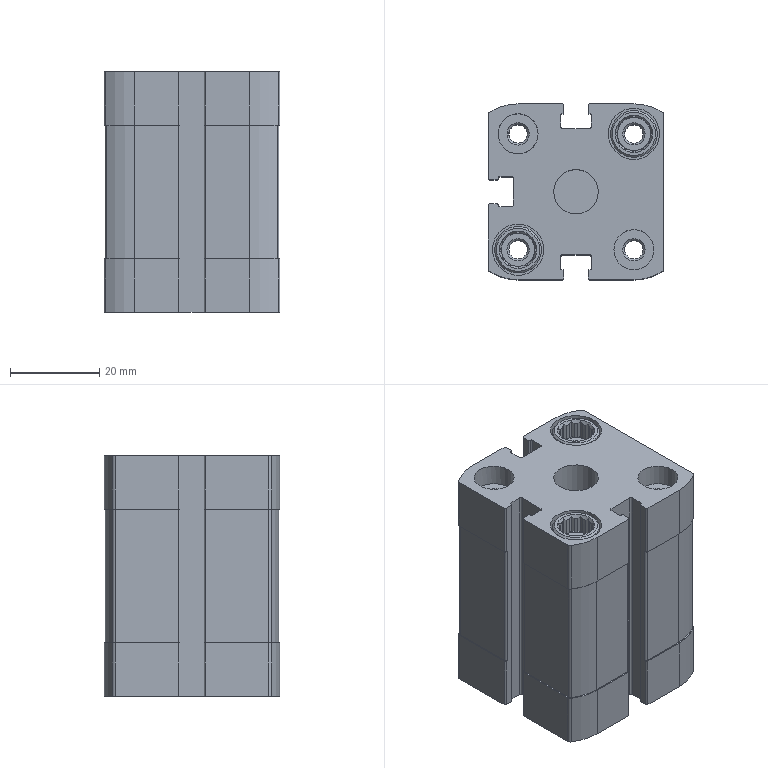Part | NX | features BREP 1 | 1 solid | 334 faces | box 39.5 x 39.5 x 54 mm | volume 58538 mm3 | plane 223 | cylinder 93 | cone 18 | commonest cylinder face diameters 0.8 x24 0.4 x12 1.6 x12 23.4 x12 4.134 x10 9 x5